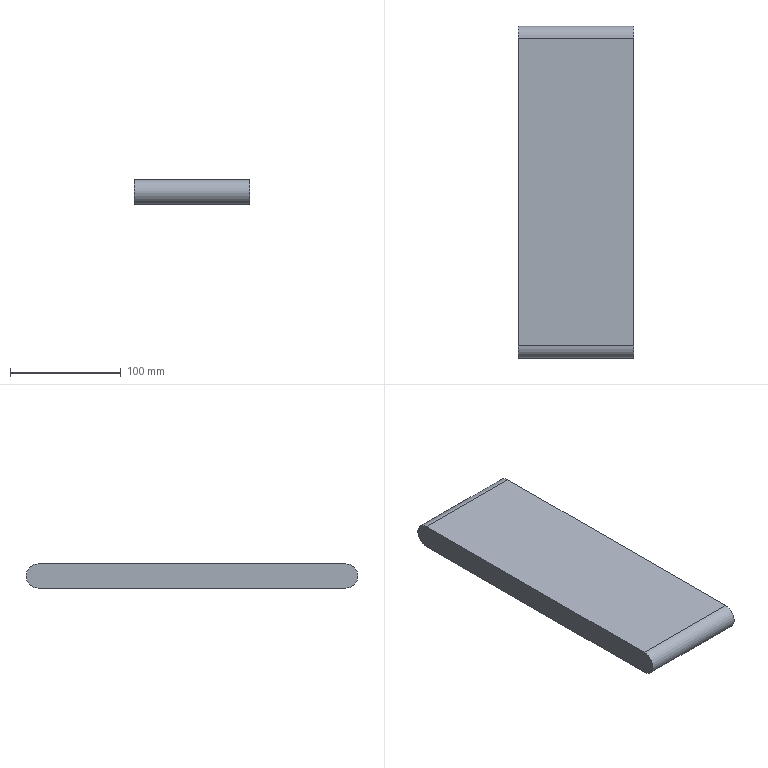Part | NX | features solid 2 | 1 solid | 6 faces | box 104 x 300.3 x 22 mm | volume 676284 mm3 | plane 4 | cylinder 2 | commonest cylinder face diameters 22 x2
STEP:
#1=CARTESIAN_POINT('',(52.,432.3,-65.5));
#2=VERTEX_POINT('',#1);
#3=CARTESIAN_POINT('',(52.,154.,-65.5));
#4=VERTEX_POINT('',#3);
#5=CARTESIAN_POINT('',(52.,315.,-65.5));
#6=DIRECTION('',(0.,-1.,0.));
#7=VECTOR('',#6,1000.);
#8=LINE('',#5,#7);
#9=EDGE_CURVE('',#2,#4,#8,.T.);
#10=ORIENTED_EDGE('',*,*,#9,.F.);
#11=CARTESIAN_POINT('',(-52.,432.3,-65.5));
#12=VERTEX_POINT('',#11);
#13=CARTESIAN_POINT('',(0.,432.3,-65.5));
#14=DIRECTION('',(1.,0.,0.));
#15=VECTOR('',#14,1000.);
#16=LINE('',#13,#15);
#17=EDGE_CURVE('',#2,#12,#16,.F.);
#18=ORIENTED_EDGE('',*,*,#17,.T.);
#19=CARTESIAN_POINT('',(-52.,154.,-65.5));
#20=VERTEX_POINT('',#19);
#21=CARTESIAN_POINT('',(-52.,315.,-65.5));
#22=DIRECTION('',(0.,1.,0.));
#23=VECTOR('',#22,1000.);
#24=LINE('',#21,#23);
#25=EDGE_CURVE('',#20,#12,#24,.T.);
#26=ORIENTED_EDGE('',*,*,#25,.F.);
#27=CARTESIAN_POINT('',(0.,154.,-65.5));
#28=DIRECTION('',(-1.,0.,0.));
#29=VECTOR('',#28,1000.);
#30=LINE('',#27,#29);
#31=EDGE_CURVE('',#20,#4,#30,.F.);
#32=ORIENTED_EDGE('',*,*,#31,.T.);
#33=EDGE_LOOP('',(#10,#18,#26,#32));
#34=FACE_BOUND('',#33,.T.);
#35=CARTESIAN_POINT('',(0.,315.,-65.5));
#36=DIRECTION('',(0.,0.,1.));
#37=DIRECTION('',(1.,0.,0.));
#38=AXIS2_PLACEMENT_3D('',#35,#36,#37);
#39=PLANE('',#38);
#40=ADVANCED_FACE('',(#34),#39,.T.);
#41=CARTESIAN_POINT('',(-52.,432.3,-87.5));
#42=VERTEX_POINT('',#41);
#43=CARTESIAN_POINT('',(-52.,432.3,-76.5));
#44=DIRECTION('',(-1.,0.,0.));
#45=DIRECTION('',(0.,0.,1.));
#46=AXIS2_PLACEMENT_3D('',#43,#44,#45);
#47=CIRCLE('',#46,11.);
#48=EDGE_CURVE('',#12,#42,#47,.T.);
#49=ORIENTED_EDGE('',*,*,#48,.T.);
#50=CARTESIAN_POINT('',(-52.,154.,-87.5));
#51=VERTEX_POINT('',#50);
#52=CARTESIAN_POINT('',(-52.,315.,-87.5));
#53=DIRECTION('',(0.,-1.,0.));
#54=VECTOR('',#53,1000.);
#55=LINE('',#52,#54);
#56=EDGE_CURVE('',#42,#51,#55,.T.);
#57=ORIENTED_EDGE('',*,*,#56,.T.);
#58=CARTESIAN_POINT('',(-52.,154.,-76.5));
#59=DIRECTION('',(-1.,0.,0.));
#60=DIRECTION('',(0.,0.,1.));
#61=AXIS2_PLACEMENT_3D('',#58,#59,#60);
#62=CIRCLE('',#61,11.);
#63=EDGE_CURVE('',#51,#20,#62,.T.);
#64=ORIENTED_EDGE('',*,*,#63,.T.);
#65=ORIENTED_EDGE('',*,*,#25,.T.);
#66=EDGE_LOOP('',(#49,#57,#64,#65));
#67=FACE_BOUND('',#66,.T.);
#68=CARTESIAN_POINT('',(-52.,315.,-87.5));
#69=DIRECTION('',(-1.,0.,0.));
#70=DIRECTION('',(0.,0.,1.));
#71=AXIS2_PLACEMENT_3D('',#68,#69,#70);
#72=PLANE('',#71);
#73=ADVANCED_FACE('',(#67),#72,.T.);
#74=ORIENTED_EDGE('',*,*,#56,.F.);
#75=CARTESIAN_POINT('',(52.,432.3,-87.5));
#76=VERTEX_POINT('',#75);
#77=CARTESIAN_POINT('',(0.,432.3,-87.5));
#78=DIRECTION('',(-1.,0.,0.));
#79=VECTOR('',#78,1000.);
#80=LINE('',#77,#79);
#81=EDGE_CURVE('',#42,#76,#80,.F.);
#82=ORIENTED_EDGE('',*,*,#81,.T.);
#83=CARTESIAN_POINT('',(52.,154.,-87.5));
#84=VERTEX_POINT('',#83);
#85=CARTESIAN_POINT('',(52.,315.,-87.5));
#86=DIRECTION('',(0.,1.,0.));
#87=VECTOR('',#86,1000.);
#88=LINE('',#85,#87);
#89=EDGE_CURVE('',#84,#76,#88,.T.);
#90=ORIENTED_EDGE('',*,*,#89,.F.);
#91=CARTESIAN_POINT('',(0.,154.,-87.5));
#92=DIRECTION('',(1.,0.,0.));
#93=VECTOR('',#92,1000.);
#94=LINE('',#91,#93);
#95=EDGE_CURVE('',#84,#51,#94,.F.);
#96=ORIENTED_EDGE('',*,*,#95,.T.);
#97=EDGE_LOOP('',(#74,#82,#90,#96));
#98=FACE_BOUND('',#97,.T.);
#99=CARTESIAN_POINT('',(0.,315.,-87.5));
#100=DIRECTION('',(0.,0.,-1.));
#101=DIRECTION('',(-1.,0.,0.));
#102=AXIS2_PLACEMENT_3D('',#99,#100,#101);
#103=PLANE('',#102);
#104=ADVANCED_FACE('',(#98),#103,.T.);
#105=ORIENTED_EDGE('',*,*,#89,.T.);
#106=CARTESIAN_POINT('',(52.,432.3,-76.5));
#107=DIRECTION('',(1.,0.,0.));
#108=DIRECTION('',(0.,0.,-1.));
#109=AXIS2_PLACEMENT_3D('',#106,#107,#108);
#110=CIRCLE('',#109,11.);
#111=EDGE_CURVE('',#76,#2,#110,.T.);
#112=ORIENTED_EDGE('',*,*,#111,.T.);
#113=ORIENTED_EDGE('',*,*,#9,.T.);
#114=CARTESIAN_POINT('',(52.,154.,-76.5));
#115=DIRECTION('',(1.,0.,0.));
#116=DIRECTION('',(0.,0.,-1.));
#117=AXIS2_PLACEMENT_3D('',#114,#115,#116);
#118=CIRCLE('',#117,11.);
#119=EDGE_CURVE('',#4,#84,#118,.T.);
#120=ORIENTED_EDGE('',*,*,#119,.T.);
#121=EDGE_LOOP('',(#105,#112,#113,#120));
#122=FACE_BOUND('',#121,.T.);
#123=CARTESIAN_POINT('',(52.,315.,-87.5));
#124=DIRECTION('',(1.,0.,0.));
#125=DIRECTION('',(0.,0.,-1.));
#126=AXIS2_PLACEMENT_3D('',#123,#124,#125);
#127=PLANE('',#126);
#128=ADVANCED_FACE('',(#122),#127,.T.);
#129=ORIENTED_EDGE('',*,*,#17,.F.);
#130=ORIENTED_EDGE('',*,*,#111,.F.);
#131=ORIENTED_EDGE('',*,*,#81,.F.);
#132=ORIENTED_EDGE('',*,*,#48,.F.);
#133=EDGE_LOOP('',(#129,#130,#131,#132));
#134=FACE_BOUND('',#133,.T.);
#135=CARTESIAN_POINT('',(-8.,432.3,-76.5));
#136=DIRECTION('',(1.,0.,0.));
#137=DIRECTION('',(0.,0.,-1.));
#138=AXIS2_PLACEMENT_3D('',#135,#136,#137);
#139=CYLINDRICAL_SURFACE('',#138,11.);
#140=ADVANCED_FACE('',(#134),#139,.T.);
#141=ORIENTED_EDGE('',*,*,#31,.F.);
#142=ORIENTED_EDGE('',*,*,#63,.F.);
#143=ORIENTED_EDGE('',*,*,#95,.F.);
#144=ORIENTED_EDGE('',*,*,#119,.F.);
#145=EDGE_LOOP('',(#141,#142,#143,#144));
#146=FACE_BOUND('',#145,.T.);
#147=CARTESIAN_POINT('',(0.,154.,-76.5));
#148=DIRECTION('',(-1.,0.,0.));
#149=DIRECTION('',(0.,0.,1.));
#150=AXIS2_PLACEMENT_3D('',#147,#148,#149);
#151=CYLINDRICAL_SURFACE('',#150,11.);
#152=ADVANCED_FACE('',(#146),#151,.T.);
#153=CLOSED_SHELL('',(#40,#73,#104,#128,#140,#152));
#154=MANIFOLD_SOLID_BREP('',#153);
#155=(LENGTH_UNIT()NAMED_UNIT(*)SI_UNIT(.MILLI.,.METRE.));
#156=UNCERTAINTY_MEASURE_WITH_UNIT(LENGTH_MEASURE(0.00001),#155,'','');
#157=(NAMED_UNIT(*)PLANE_ANGLE_UNIT()SI_UNIT($,.RADIAN.));
#158=(NAMED_UNIT(*)SI_UNIT($,.STERADIAN.)SOLID_ANGLE_UNIT());
#159=(GEOMETRIC_REPRESENTATION_CONTEXT(3)GLOBAL_UNCERTAINTY_ASSIGNED_CONTEXT((#156))GLOBAL_UNIT_ASSIGNED_CONTEXT((#155,#157,#158))REPRESENTATION_CONTEXT('',''));
#160=ADVANCED_BREP_SHAPE_REPRESENTATION('',(#154),#159);